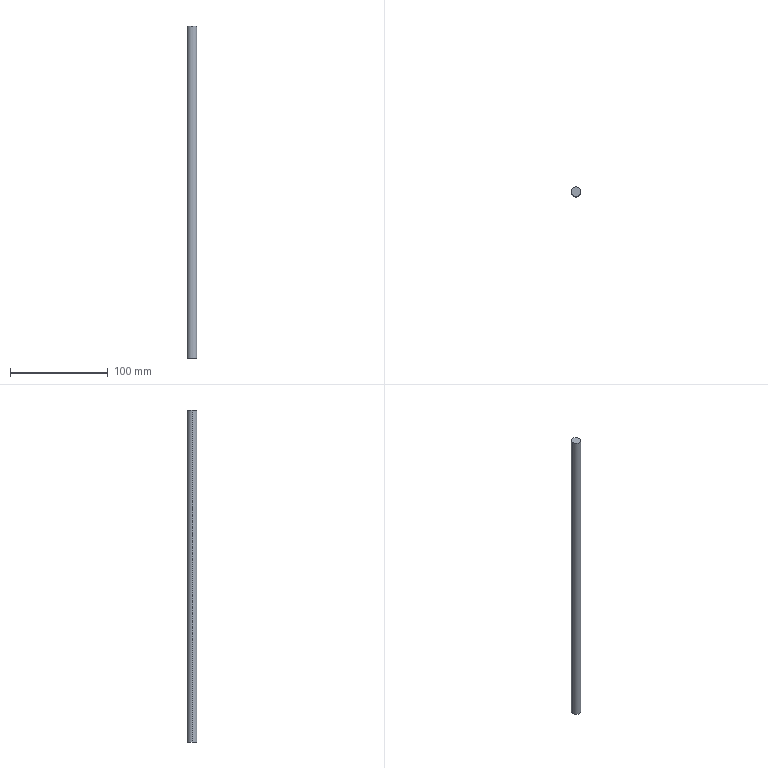Part | STEP file | 1 solid | 4 faces | box 10 x 10 x 340 mm | volume 26704 mm3 | cylinder 2 | plane 2 | commonest cylinder face diameters 10 x2
STEP:
#1=CARTESIAN_POINT('',(0.,0.,0.));
#2=DIRECTION('',(0.,0.,1.));
#3=DIRECTION('',(1.,0.,0.));
#4=AXIS2_PLACEMENT_3D('',#1,#2,#3);
#5=CARTESIAN_POINT('',(5.,0.,340.));
#6=VERTEX_POINT('',#5);
#7=CARTESIAN_POINT('',(-5.,0.,340.));
#8=VERTEX_POINT('',#7);
#9=CARTESIAN_POINT('',(0.,0.,340.));
#10=DIRECTION('',(0.,0.,1.));
#11=DIRECTION('',(1.,0.,0.));
#12=AXIS2_PLACEMENT_3D('',#9,#10,#11);
#13=CIRCLE('',#12,5.);
#14=CARTESIAN_POINT('',(0.,0.,340.));
#15=DIRECTION('',(0.,0.,-1.));
#16=DIRECTION('',(-1.,0.,0.));
#17=AXIS2_PLACEMENT_3D('',#14,#15,#16);
#18=CYLINDRICAL_SURFACE('',#17,5.);
#19=CARTESIAN_POINT('',(3.142,0.));
#20=DIRECTION('',(-1.,0.));
#21=VECTOR('',#20,1.);
#22=LINE('',#19,#21);
#23=(GEOMETRIC_REPRESENTATION_CONTEXT(2)PARAMETRIC_REPRESENTATION_CONTEXT()REPRESENTATION_CONTEXT('',''));
#24=DEFINITIONAL_REPRESENTATION('',(#22),#23);
#25=PCURVE('',#18,#24);
#26=CARTESIAN_POINT('',(0.,0.,340.));
#27=DIRECTION('',(0.,0.,1.));
#28=DIRECTION('',(1.,0.,0.));
#29=AXIS2_PLACEMENT_3D('',#26,#27,#28);
#30=PLANE('',#29);
#31=CARTESIAN_POINT('',(0.,0.));
#32=DIRECTION('',(1.,0.));
#33=AXIS2_PLACEMENT_2D('',#31,#32);
#34=CIRCLE('',#33,5.);
#35=(GEOMETRIC_REPRESENTATION_CONTEXT(2)PARAMETRIC_REPRESENTATION_CONTEXT()REPRESENTATION_CONTEXT('',''));
#36=DEFINITIONAL_REPRESENTATION('',(#34),#35);
#37=PCURVE('',#30,#36);
#38=SURFACE_CURVE('',#13,(#25,#37),.PCURVE_S1.);
#39=EDGE_CURVE('',#6,#8,#38,.T.);
#40=ORIENTED_EDGE('',*,*,#39,.F.);
#41=CARTESIAN_POINT('',(5.,0.,0.));
#42=VERTEX_POINT('',#41);
#43=CARTESIAN_POINT('',(5.,0.,340.));
#44=DIRECTION('',(0.,0.,-1.));
#45=VECTOR('',#44,1.);
#46=LINE('',#43,#45);
#47=CARTESIAN_POINT('',(3.142,0.));
#48=DIRECTION('',(0.,1.));
#49=VECTOR('',#48,1.);
#50=LINE('',#47,#49);
#51=(GEOMETRIC_REPRESENTATION_CONTEXT(2)PARAMETRIC_REPRESENTATION_CONTEXT()REPRESENTATION_CONTEXT('',''));
#52=DEFINITIONAL_REPRESENTATION('',(#50),#51);
#53=PCURVE('',#18,#52);
#54=CARTESIAN_POINT('',(0.,0.,340.));
#55=DIRECTION('',(0.,0.,-1.));
#56=DIRECTION('',(-1.,0.,0.));
#57=AXIS2_PLACEMENT_3D('',#54,#55,#56);
#58=CYLINDRICAL_SURFACE('',#57,5.);
#59=CARTESIAN_POINT('',(3.142,0.));
#60=DIRECTION('',(0.,1.));
#61=VECTOR('',#60,1.);
#62=LINE('',#59,#61);
#63=(GEOMETRIC_REPRESENTATION_CONTEXT(2)PARAMETRIC_REPRESENTATION_CONTEXT()REPRESENTATION_CONTEXT('',''));
#64=DEFINITIONAL_REPRESENTATION('',(#62),#63);
#65=PCURVE('',#58,#64);
#66=SURFACE_CURVE('',#46,(#53,#65),.PCURVE_S1.);
#67=EDGE_CURVE('',#6,#42,#66,.T.);
#68=ORIENTED_EDGE('',*,*,#67,.T.);
#69=CARTESIAN_POINT('',(-5.,0.,0.));
#70=VERTEX_POINT('',#69);
#71=CARTESIAN_POINT('',(0.,0.,0.));
#72=DIRECTION('',(0.,0.,1.));
#73=DIRECTION('',(1.,0.,0.));
#74=AXIS2_PLACEMENT_3D('',#71,#72,#73);
#75=CIRCLE('',#74,5.);
#76=CARTESIAN_POINT('',(3.142,340.));
#77=DIRECTION('',(-1.,0.));
#78=VECTOR('',#77,1.);
#79=LINE('',#76,#78);
#80=(GEOMETRIC_REPRESENTATION_CONTEXT(2)PARAMETRIC_REPRESENTATION_CONTEXT()REPRESENTATION_CONTEXT('',''));
#81=DEFINITIONAL_REPRESENTATION('',(#79),#80);
#82=PCURVE('',#18,#81);
#83=CARTESIAN_POINT('',(0.,0.,0.));
#84=DIRECTION('',(0.,0.,1.));
#85=DIRECTION('',(1.,0.,0.));
#86=AXIS2_PLACEMENT_3D('',#83,#84,#85);
#87=PLANE('',#86);
#88=CARTESIAN_POINT('',(0.,0.));
#89=DIRECTION('',(1.,0.));
#90=AXIS2_PLACEMENT_2D('',#88,#89);
#91=CIRCLE('',#90,5.);
#92=(GEOMETRIC_REPRESENTATION_CONTEXT(2)PARAMETRIC_REPRESENTATION_CONTEXT()REPRESENTATION_CONTEXT('',''));
#93=DEFINITIONAL_REPRESENTATION('',(#91),#92);
#94=PCURVE('',#87,#93);
#95=SURFACE_CURVE('',#75,(#82,#94),.PCURVE_S1.);
#96=EDGE_CURVE('',#42,#70,#95,.T.);
#97=ORIENTED_EDGE('',*,*,#96,.T.);
#98=CARTESIAN_POINT('',(-5.,0.,340.));
#99=DIRECTION('',(0.,0.,-1.));
#100=VECTOR('',#99,1.);
#101=LINE('',#98,#100);
#102=CARTESIAN_POINT('',(0.,0.));
#103=DIRECTION('',(0.,1.));
#104=VECTOR('',#103,1.);
#105=LINE('',#102,#104);
#106=(GEOMETRIC_REPRESENTATION_CONTEXT(2)PARAMETRIC_REPRESENTATION_CONTEXT()REPRESENTATION_CONTEXT('',''));
#107=DEFINITIONAL_REPRESENTATION('',(#105),#106);
#108=PCURVE('',#18,#107);
#109=CARTESIAN_POINT('',(6.283,0.));
#110=DIRECTION('',(0.,1.));
#111=VECTOR('',#110,1.);
#112=LINE('',#109,#111);
#113=(GEOMETRIC_REPRESENTATION_CONTEXT(2)PARAMETRIC_REPRESENTATION_CONTEXT()REPRESENTATION_CONTEXT('',''));
#114=DEFINITIONAL_REPRESENTATION('',(#112),#113);
#115=PCURVE('',#58,#114);
#116=SURFACE_CURVE('',#101,(#108,#115),.PCURVE_S1.);
#117=EDGE_CURVE('',#8,#70,#116,.T.);
#118=ORIENTED_EDGE('',*,*,#117,.F.);
#119=EDGE_LOOP('',(#40,#68,#97,#118));
#120=FACE_BOUND('',#119,.T.);
#121=ADVANCED_FACE('',(#120),#18,.T.);
#122=ORIENTED_EDGE('',*,*,#67,.F.);
#123=CARTESIAN_POINT('',(0.,0.,340.));
#124=DIRECTION('',(0.,0.,1.));
#125=DIRECTION('',(1.,0.,0.));
#126=AXIS2_PLACEMENT_3D('',#123,#124,#125);
#127=CIRCLE('',#126,5.);
#128=CARTESIAN_POINT('',(9.425,0.));
#129=DIRECTION('',(-1.,0.));
#130=VECTOR('',#129,1.);
#131=LINE('',#128,#130);
#132=(GEOMETRIC_REPRESENTATION_CONTEXT(2)PARAMETRIC_REPRESENTATION_CONTEXT()REPRESENTATION_CONTEXT('',''));
#133=DEFINITIONAL_REPRESENTATION('',(#131),#132);
#134=PCURVE('',#58,#133);
#135=CARTESIAN_POINT('',(0.,0.));
#136=DIRECTION('',(1.,0.));
#137=AXIS2_PLACEMENT_2D('',#135,#136);
#138=CIRCLE('',#137,5.);
#139=(GEOMETRIC_REPRESENTATION_CONTEXT(2)PARAMETRIC_REPRESENTATION_CONTEXT()REPRESENTATION_CONTEXT('',''));
#140=DEFINITIONAL_REPRESENTATION('',(#138),#139);
#141=PCURVE('',#30,#140);
#142=SURFACE_CURVE('',#127,(#134,#141),.PCURVE_S1.);
#143=EDGE_CURVE('',#8,#6,#142,.T.);
#144=ORIENTED_EDGE('',*,*,#143,.F.);
#145=ORIENTED_EDGE('',*,*,#117,.T.);
#146=CARTESIAN_POINT('',(0.,0.,0.));
#147=DIRECTION('',(0.,0.,1.));
#148=DIRECTION('',(1.,0.,0.));
#149=AXIS2_PLACEMENT_3D('',#146,#147,#148);
#150=CIRCLE('',#149,5.);
#151=CARTESIAN_POINT('',(9.425,340.));
#152=DIRECTION('',(-1.,0.));
#153=VECTOR('',#152,1.);
#154=LINE('',#151,#153);
#155=(GEOMETRIC_REPRESENTATION_CONTEXT(2)PARAMETRIC_REPRESENTATION_CONTEXT()REPRESENTATION_CONTEXT('',''));
#156=DEFINITIONAL_REPRESENTATION('',(#154),#155);
#157=PCURVE('',#58,#156);
#158=CARTESIAN_POINT('',(0.,0.));
#159=DIRECTION('',(1.,0.));
#160=AXIS2_PLACEMENT_2D('',#158,#159);
#161=CIRCLE('',#160,5.);
#162=(GEOMETRIC_REPRESENTATION_CONTEXT(2)PARAMETRIC_REPRESENTATION_CONTEXT()REPRESENTATION_CONTEXT('',''));
#163=DEFINITIONAL_REPRESENTATION('',(#161),#162);
#164=PCURVE('',#87,#163);
#165=SURFACE_CURVE('',#150,(#157,#164),.PCURVE_S1.);
#166=EDGE_CURVE('',#70,#42,#165,.T.);
#167=ORIENTED_EDGE('',*,*,#166,.T.);
#168=EDGE_LOOP('',(#122,#144,#145,#167));
#169=FACE_BOUND('',#168,.T.);
#170=ADVANCED_FACE('',(#169),#58,.T.);
#171=ORIENTED_EDGE('',*,*,#143,.T.);
#172=ORIENTED_EDGE('',*,*,#39,.T.);
#173=EDGE_LOOP('',(#171,#172));
#174=FACE_BOUND('',#173,.T.);
#175=ADVANCED_FACE('',(#174),#30,.T.);
#176=ORIENTED_EDGE('',*,*,#166,.F.);
#177=ORIENTED_EDGE('',*,*,#96,.F.);
#178=EDGE_LOOP('',(#176,#177));
#179=FACE_BOUND('',#178,.T.);
#180=ADVANCED_FACE('',(#179),#87,.F.);
#181=CLOSED_SHELL('',(#121,#170,#175,#180));
#182=MANIFOLD_SOLID_BREP('',#181);
#183=(LENGTH_UNIT()NAMED_UNIT(*)SI_UNIT(.MILLI.,.METRE.));
#184=UNCERTAINTY_MEASURE_WITH_UNIT(LENGTH_MEASURE(0.0000001),#183,'','');
#185=(NAMED_UNIT(*)PLANE_ANGLE_UNIT()SI_UNIT($,.RADIAN.));
#186=(NAMED_UNIT(*)SI_UNIT($,.STERADIAN.)SOLID_ANGLE_UNIT());
#187=(GEOMETRIC_REPRESENTATION_CONTEXT(3)GLOBAL_UNCERTAINTY_ASSIGNED_CONTEXT((#184))GLOBAL_UNIT_ASSIGNED_CONTEXT((#183,#185,#186))REPRESENTATION_CONTEXT('',''));
#188=ADVANCED_BREP_SHAPE_REPRESENTATION('',(#4,#182),#187);